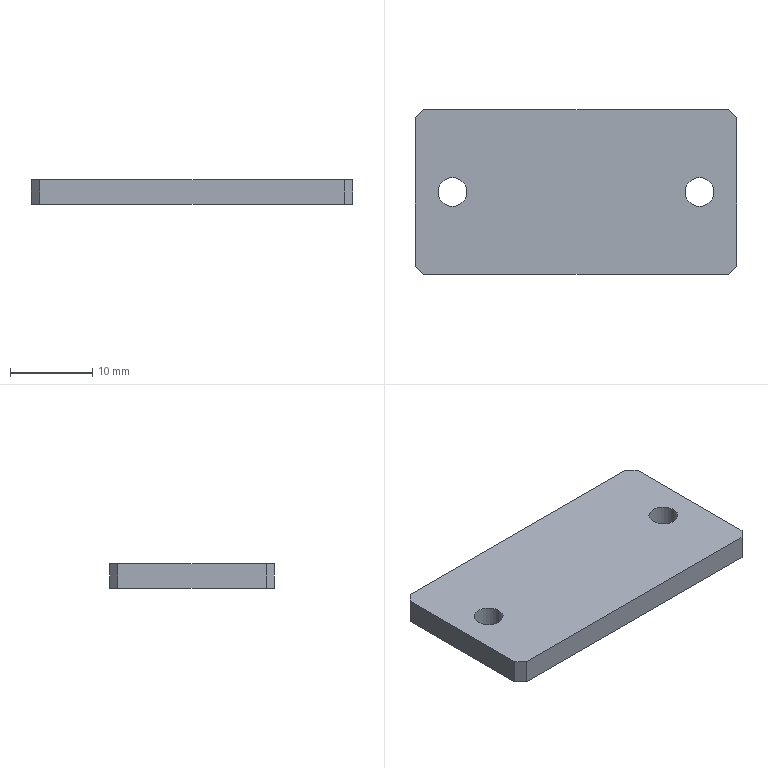Part | SolidWorks | features Chamfer 1, Extrusion 1 | 1 solid | 14 faces | box 39 x 20 x 3 mm | volume 2276 mm3 | plane 10 | cylinder 4 | commonest cylinder face diameters 3.5 x4
STEP:
#1=CARTESIAN_POINT('',(13.25,0.,3.));
#2=VERTEX_POINT('',#1);
#3=CARTESIAN_POINT('',(16.75,0.,3.));
#4=VERTEX_POINT('',#3);
#5=CARTESIAN_POINT('',(15.,0.,3.));
#6=DIRECTION('',(0.,0.,1.));
#7=DIRECTION('',(1.,0.,0.));
#8=AXIS2_PLACEMENT_3D('',#5,#6,#7);
#9=CIRCLE('',#8,1.75);
#10=EDGE_CURVE('',#2,#4,#9,.T.);
#11=ORIENTED_EDGE('',*,*,#10,.T.);
#12=CARTESIAN_POINT('',(16.75,0.,0.));
#13=VERTEX_POINT('',#12);
#14=CARTESIAN_POINT('',(16.75,0.,3.));
#15=DIRECTION('',(0.,0.,-1.));
#16=VECTOR('',#15,1000.);
#17=LINE('',#14,#16);
#18=EDGE_CURVE('',#4,#13,#17,.T.);
#19=ORIENTED_EDGE('',*,*,#18,.T.);
#20=CARTESIAN_POINT('',(13.25,0.,0.));
#21=VERTEX_POINT('',#20);
#22=CARTESIAN_POINT('',(15.,0.,0.));
#23=DIRECTION('',(0.,0.,1.));
#24=DIRECTION('',(1.,0.,0.));
#25=AXIS2_PLACEMENT_3D('',#22,#23,#24);
#26=CIRCLE('',#25,1.75);
#27=EDGE_CURVE('',#21,#13,#26,.T.);
#28=ORIENTED_EDGE('',*,*,#27,.F.);
#29=CARTESIAN_POINT('',(13.25,0.,3.));
#30=DIRECTION('',(0.,0.,-1.));
#31=VECTOR('',#30,1000.);
#32=LINE('',#29,#31);
#33=EDGE_CURVE('',#2,#21,#32,.T.);
#34=ORIENTED_EDGE('',*,*,#33,.F.);
#35=EDGE_LOOP('',(#11,#19,#28,#34));
#36=FACE_OUTER_BOUND('',#35,.T.);
#37=CARTESIAN_POINT('',(15.,0.,3.));
#38=DIRECTION('',(0.,0.,-1.));
#39=DIRECTION('',(-1.,0.,0.));
#40=AXIS2_PLACEMENT_3D('',#37,#38,#39);
#41=CYLINDRICAL_SURFACE('',#40,1.75);
#42=ADVANCED_FACE('',(#36),#41,.F.);
#43=CARTESIAN_POINT('',(-16.75,0.,3.));
#44=VERTEX_POINT('',#43);
#45=CARTESIAN_POINT('',(-13.25,0.,3.));
#46=VERTEX_POINT('',#45);
#47=CARTESIAN_POINT('',(-15.,0.,3.));
#48=DIRECTION('',(0.,0.,1.));
#49=DIRECTION('',(1.,0.,0.));
#50=AXIS2_PLACEMENT_3D('',#47,#48,#49);
#51=CIRCLE('',#50,1.75);
#52=EDGE_CURVE('',#44,#46,#51,.T.);
#53=ORIENTED_EDGE('',*,*,#52,.T.);
#54=CARTESIAN_POINT('',(-13.25,0.,0.));
#55=VERTEX_POINT('',#54);
#56=CARTESIAN_POINT('',(-13.25,0.,3.));
#57=DIRECTION('',(0.,0.,-1.));
#58=VECTOR('',#57,1000.);
#59=LINE('',#56,#58);
#60=EDGE_CURVE('',#46,#55,#59,.T.);
#61=ORIENTED_EDGE('',*,*,#60,.T.);
#62=CARTESIAN_POINT('',(-16.75,0.,0.));
#63=VERTEX_POINT('',#62);
#64=CARTESIAN_POINT('',(-15.,0.,0.));
#65=DIRECTION('',(0.,0.,1.));
#66=DIRECTION('',(1.,0.,0.));
#67=AXIS2_PLACEMENT_3D('',#64,#65,#66);
#68=CIRCLE('',#67,1.75);
#69=EDGE_CURVE('',#63,#55,#68,.T.);
#70=ORIENTED_EDGE('',*,*,#69,.F.);
#71=CARTESIAN_POINT('',(-16.75,0.,3.));
#72=DIRECTION('',(0.,0.,-1.));
#73=VECTOR('',#72,1000.);
#74=LINE('',#71,#73);
#75=EDGE_CURVE('',#44,#63,#74,.T.);
#76=ORIENTED_EDGE('',*,*,#75,.F.);
#77=EDGE_LOOP('',(#53,#61,#70,#76));
#78=FACE_OUTER_BOUND('',#77,.T.);
#79=CARTESIAN_POINT('',(-15.,0.,3.));
#80=DIRECTION('',(0.,0.,-1.));
#81=DIRECTION('',(-1.,0.,0.));
#82=AXIS2_PLACEMENT_3D('',#79,#80,#81);
#83=CYLINDRICAL_SURFACE('',#82,1.75);
#84=ADVANCED_FACE('',(#78),#83,.F.);
#85=CARTESIAN_POINT('',(-18.5,-10.,3.));
#86=VERTEX_POINT('',#85);
#87=CARTESIAN_POINT('',(18.5,-10.,3.));
#88=VERTEX_POINT('',#87);
#89=CARTESIAN_POINT('',(-19.5,-10.,3.));
#90=DIRECTION('',(1.,0.,0.));
#91=VECTOR('',#90,1000.);
#92=LINE('',#89,#91);
#93=EDGE_CURVE('',#86,#88,#92,.T.);
#94=ORIENTED_EDGE('',*,*,#93,.T.);
#95=CARTESIAN_POINT('',(19.5,-9.,3.));
#96=VERTEX_POINT('',#95);
#97=CARTESIAN_POINT('',(19.5,-9.,3.));
#98=DIRECTION('',(0.7071,0.7071,0.));
#99=VECTOR('',#98,1000.);
#100=LINE('',#97,#99);
#101=EDGE_CURVE('',#88,#96,#100,.T.);
#102=ORIENTED_EDGE('',*,*,#101,.T.);
#103=CARTESIAN_POINT('',(19.5,9.,3.));
#104=VERTEX_POINT('',#103);
#105=CARTESIAN_POINT('',(19.5,-10.,3.));
#106=DIRECTION('',(0.,1.,0.));
#107=VECTOR('',#106,1000.);
#108=LINE('',#105,#107);
#109=EDGE_CURVE('',#96,#104,#108,.T.);
#110=ORIENTED_EDGE('',*,*,#109,.T.);
#111=CARTESIAN_POINT('',(18.5,10.,3.));
#112=VERTEX_POINT('',#111);
#113=CARTESIAN_POINT('',(18.5,10.,3.));
#114=DIRECTION('',(-0.7071,0.7071,0.));
#115=VECTOR('',#114,1000.);
#116=LINE('',#113,#115);
#117=EDGE_CURVE('',#104,#112,#116,.T.);
#118=ORIENTED_EDGE('',*,*,#117,.T.);
#119=CARTESIAN_POINT('',(-18.5,10.,3.));
#120=VERTEX_POINT('',#119);
#121=CARTESIAN_POINT('',(-19.5,10.,3.));
#122=DIRECTION('',(-1.,0.,0.));
#123=VECTOR('',#122,1000.);
#124=LINE('',#121,#123);
#125=EDGE_CURVE('',#112,#120,#124,.T.);
#126=ORIENTED_EDGE('',*,*,#125,.T.);
#127=CARTESIAN_POINT('',(-19.5,9.,3.));
#128=VERTEX_POINT('',#127);
#129=CARTESIAN_POINT('',(-19.5,9.,3.));
#130=DIRECTION('',(-0.7071,-0.7071,0.));
#131=VECTOR('',#130,1000.);
#132=LINE('',#129,#131);
#133=EDGE_CURVE('',#120,#128,#132,.T.);
#134=ORIENTED_EDGE('',*,*,#133,.T.);
#135=CARTESIAN_POINT('',(-19.5,-9.,3.));
#136=VERTEX_POINT('',#135);
#137=CARTESIAN_POINT('',(-19.5,-10.,3.));
#138=DIRECTION('',(0.,-1.,0.));
#139=VECTOR('',#138,1000.);
#140=LINE('',#137,#139);
#141=EDGE_CURVE('',#128,#136,#140,.T.);
#142=ORIENTED_EDGE('',*,*,#141,.T.);
#143=CARTESIAN_POINT('',(-18.5,-10.,3.));
#144=DIRECTION('',(0.7071,-0.7071,0.));
#145=VECTOR('',#144,1000.);
#146=LINE('',#143,#145);
#147=EDGE_CURVE('',#136,#86,#146,.T.);
#148=ORIENTED_EDGE('',*,*,#147,.T.);
#149=EDGE_LOOP('',(#94,#102,#110,#118,#126,#134,#142,#148));
#150=FACE_OUTER_BOUND('',#149,.T.);
#151=ORIENTED_EDGE('',*,*,#52,.F.);
#152=CARTESIAN_POINT('',(-15.,0.,3.));
#153=DIRECTION('',(0.,0.,1.));
#154=DIRECTION('',(1.,0.,0.));
#155=AXIS2_PLACEMENT_3D('',#152,#153,#154);
#156=CIRCLE('',#155,1.75);
#157=EDGE_CURVE('',#46,#44,#156,.T.);
#158=ORIENTED_EDGE('',*,*,#157,.F.);
#159=EDGE_LOOP('',(#151,#158));
#160=FACE_BOUND('',#159,.T.);
#161=ORIENTED_EDGE('',*,*,#10,.F.);
#162=CARTESIAN_POINT('',(15.,0.,3.));
#163=DIRECTION('',(0.,0.,1.));
#164=DIRECTION('',(1.,0.,0.));
#165=AXIS2_PLACEMENT_3D('',#162,#163,#164);
#166=CIRCLE('',#165,1.75);
#167=EDGE_CURVE('',#4,#2,#166,.T.);
#168=ORIENTED_EDGE('',*,*,#167,.F.);
#169=EDGE_LOOP('',(#161,#168));
#170=FACE_BOUND('',#169,.T.);
#171=CARTESIAN_POINT('',(0.,0.,3.));
#172=DIRECTION('',(0.,0.,-1.));
#173=DIRECTION('',(-1.,0.,0.));
#174=AXIS2_PLACEMENT_3D('',#171,#172,#173);
#175=PLANE('',#174);
#176=ADVANCED_FACE('',(#150,#160,#170),#175,.F.);
#177=ORIENTED_EDGE('',*,*,#69,.T.);
#178=CARTESIAN_POINT('',(-15.,0.,0.));
#179=DIRECTION('',(0.,0.,1.));
#180=DIRECTION('',(1.,0.,0.));
#181=AXIS2_PLACEMENT_3D('',#178,#179,#180);
#182=CIRCLE('',#181,1.75);
#183=EDGE_CURVE('',#55,#63,#182,.T.);
#184=ORIENTED_EDGE('',*,*,#183,.T.);
#185=EDGE_LOOP('',(#177,#184));
#186=FACE_BOUND('',#185,.T.);
#187=CARTESIAN_POINT('',(19.5,-9.,0.));
#188=VERTEX_POINT('',#187);
#189=CARTESIAN_POINT('',(19.5,9.,0.));
#190=VERTEX_POINT('',#189);
#191=CARTESIAN_POINT('',(19.5,-10.,0.));
#192=DIRECTION('',(0.,1.,0.));
#193=VECTOR('',#192,1000.);
#194=LINE('',#191,#193);
#195=EDGE_CURVE('',#188,#190,#194,.T.);
#196=ORIENTED_EDGE('',*,*,#195,.F.);
#197=CARTESIAN_POINT('',(18.5,-10.,0.));
#198=VERTEX_POINT('',#197);
#199=CARTESIAN_POINT('',(14.25,-14.25,0.));
#200=DIRECTION('',(-0.7071,-0.7071,0.));
#201=VECTOR('',#200,1000.);
#202=LINE('',#199,#201);
#203=EDGE_CURVE('',#188,#198,#202,.T.);
#204=ORIENTED_EDGE('',*,*,#203,.T.);
#205=CARTESIAN_POINT('',(-18.5,-10.,0.));
#206=VERTEX_POINT('',#205);
#207=CARTESIAN_POINT('',(-19.5,-10.,0.));
#208=DIRECTION('',(1.,0.,0.));
#209=VECTOR('',#208,1000.);
#210=LINE('',#207,#209);
#211=EDGE_CURVE('',#206,#198,#210,.T.);
#212=ORIENTED_EDGE('',*,*,#211,.F.);
#213=CARTESIAN_POINT('',(-19.5,-9.,0.));
#214=VERTEX_POINT('',#213);
#215=CARTESIAN_POINT('',(-14.25,-14.25,0.));
#216=DIRECTION('',(-0.7071,0.7071,0.));
#217=VECTOR('',#216,1000.);
#218=LINE('',#215,#217);
#219=EDGE_CURVE('',#206,#214,#218,.T.);
#220=ORIENTED_EDGE('',*,*,#219,.T.);
#221=CARTESIAN_POINT('',(-19.5,9.,0.));
#222=VERTEX_POINT('',#221);
#223=CARTESIAN_POINT('',(-19.5,-10.,0.));
#224=DIRECTION('',(0.,-1.,0.));
#225=VECTOR('',#224,1000.);
#226=LINE('',#223,#225);
#227=EDGE_CURVE('',#222,#214,#226,.T.);
#228=ORIENTED_EDGE('',*,*,#227,.F.);
#229=CARTESIAN_POINT('',(-18.5,10.,0.));
#230=VERTEX_POINT('',#229);
#231=CARTESIAN_POINT('',(-14.25,14.25,0.));
#232=DIRECTION('',(0.7071,0.7071,0.));
#233=VECTOR('',#232,1000.);
#234=LINE('',#231,#233);
#235=EDGE_CURVE('',#222,#230,#234,.T.);
#236=ORIENTED_EDGE('',*,*,#235,.T.);
#237=CARTESIAN_POINT('',(18.5,10.,0.));
#238=VERTEX_POINT('',#237);
#239=CARTESIAN_POINT('',(-19.5,10.,0.));
#240=DIRECTION('',(-1.,0.,0.));
#241=VECTOR('',#240,1000.);
#242=LINE('',#239,#241);
#243=EDGE_CURVE('',#238,#230,#242,.T.);
#244=ORIENTED_EDGE('',*,*,#243,.F.);
#245=CARTESIAN_POINT('',(14.25,14.25,0.));
#246=DIRECTION('',(0.7071,-0.7071,0.));
#247=VECTOR('',#246,1000.);
#248=LINE('',#245,#247);
#249=EDGE_CURVE('',#238,#190,#248,.T.);
#250=ORIENTED_EDGE('',*,*,#249,.T.);
#251=EDGE_LOOP('',(#196,#204,#212,#220,#228,#236,#244,#250));
#252=FACE_OUTER_BOUND('',#251,.T.);
#253=ORIENTED_EDGE('',*,*,#27,.T.);
#254=CARTESIAN_POINT('',(15.,0.,0.));
#255=DIRECTION('',(0.,0.,1.));
#256=DIRECTION('',(1.,0.,0.));
#257=AXIS2_PLACEMENT_3D('',#254,#255,#256);
#258=CIRCLE('',#257,1.75);
#259=EDGE_CURVE('',#13,#21,#258,.T.);
#260=ORIENTED_EDGE('',*,*,#259,.T.);
#261=EDGE_LOOP('',(#253,#260));
#262=FACE_BOUND('',#261,.T.);
#263=CARTESIAN_POINT('',(0.,0.,0.));
#264=DIRECTION('',(0.,0.,-1.));
#265=DIRECTION('',(-1.,0.,0.));
#266=AXIS2_PLACEMENT_3D('',#263,#264,#265);
#267=PLANE('',#266);
#268=ADVANCED_FACE('',(#186,#252,#262),#267,.T.);
#269=ORIENTED_EDGE('',*,*,#109,.F.);
#270=CARTESIAN_POINT('',(19.5,-9.,3.));
#271=DIRECTION('',(0.,0.,-1.));
#272=VECTOR('',#271,1000.);
#273=LINE('',#270,#272);
#274=EDGE_CURVE('',#96,#188,#273,.T.);
#275=ORIENTED_EDGE('',*,*,#274,.T.);
#276=ORIENTED_EDGE('',*,*,#195,.T.);
#277=CARTESIAN_POINT('',(19.5,9.,3.));
#278=DIRECTION('',(0.,0.,1.));
#279=VECTOR('',#278,1000.);
#280=LINE('',#277,#279);
#281=EDGE_CURVE('',#190,#104,#280,.T.);
#282=ORIENTED_EDGE('',*,*,#281,.T.);
#283=EDGE_LOOP('',(#269,#275,#276,#282));
#284=FACE_OUTER_BOUND('',#283,.T.);
#285=CARTESIAN_POINT('',(19.5,-10.,3.));
#286=DIRECTION('',(-1.,0.,0.));
#287=DIRECTION('',(0.,-1.,0.));
#288=AXIS2_PLACEMENT_3D('',#285,#286,#287);
#289=PLANE('',#288);
#290=ADVANCED_FACE('',(#284),#289,.F.);
#291=ORIENTED_EDGE('',*,*,#125,.F.);
#292=CARTESIAN_POINT('',(18.5,10.,3.));
#293=DIRECTION('',(0.,0.,-1.));
#294=VECTOR('',#293,1000.);
#295=LINE('',#292,#294);
#296=EDGE_CURVE('',#112,#238,#295,.T.);
#297=ORIENTED_EDGE('',*,*,#296,.T.);
#298=ORIENTED_EDGE('',*,*,#243,.T.);
#299=CARTESIAN_POINT('',(-18.5,10.,3.));
#300=DIRECTION('',(0.,0.,1.));
#301=VECTOR('',#300,1000.);
#302=LINE('',#299,#301);
#303=EDGE_CURVE('',#230,#120,#302,.T.);
#304=ORIENTED_EDGE('',*,*,#303,.T.);
#305=EDGE_LOOP('',(#291,#297,#298,#304));
#306=FACE_OUTER_BOUND('',#305,.T.);
#307=CARTESIAN_POINT('',(-19.5,10.,3.));
#308=DIRECTION('',(0.,-1.,0.));
#309=DIRECTION('',(1.,0.,0.));
#310=AXIS2_PLACEMENT_3D('',#307,#308,#309);
#311=PLANE('',#310);
#312=ADVANCED_FACE('',(#306),#311,.F.);
#313=ORIENTED_EDGE('',*,*,#227,.T.);
#314=CARTESIAN_POINT('',(-19.5,-9.,3.));
#315=DIRECTION('',(0.,0.,1.));
#316=VECTOR('',#315,1000.);
#317=LINE('',#314,#316);
#318=EDGE_CURVE('',#214,#136,#317,.T.);
#319=ORIENTED_EDGE('',*,*,#318,.T.);
#320=ORIENTED_EDGE('',*,*,#141,.F.);
#321=CARTESIAN_POINT('',(-19.5,9.,3.));
#322=DIRECTION('',(0.,0.,-1.));
#323=VECTOR('',#322,1000.);
#324=LINE('',#321,#323);
#325=EDGE_CURVE('',#128,#222,#324,.T.);
#326=ORIENTED_EDGE('',*,*,#325,.T.);
#327=EDGE_LOOP('',(#313,#319,#320,#326));
#328=FACE_OUTER_BOUND('',#327,.T.);
#329=CARTESIAN_POINT('',(-19.5,-10.,3.));
#330=DIRECTION('',(1.,0.,0.));
#331=DIRECTION('',(0.,0.,-1.));
#332=AXIS2_PLACEMENT_3D('',#329,#330,#331);
#333=PLANE('',#332);
#334=ADVANCED_FACE('',(#328),#333,.F.);
#335=ORIENTED_EDGE('',*,*,#211,.T.);
#336=CARTESIAN_POINT('',(18.5,-10.,3.));
#337=DIRECTION('',(0.,0.,1.));
#338=VECTOR('',#337,1000.);
#339=LINE('',#336,#338);
#340=EDGE_CURVE('',#198,#88,#339,.T.);
#341=ORIENTED_EDGE('',*,*,#340,.T.);
#342=ORIENTED_EDGE('',*,*,#93,.F.);
#343=CARTESIAN_POINT('',(-18.5,-10.,3.));
#344=DIRECTION('',(0.,0.,-1.));
#345=VECTOR('',#344,1000.);
#346=LINE('',#343,#345);
#347=EDGE_CURVE('',#86,#206,#346,.T.);
#348=ORIENTED_EDGE('',*,*,#347,.T.);
#349=EDGE_LOOP('',(#335,#341,#342,#348));
#350=FACE_OUTER_BOUND('',#349,.T.);
#351=CARTESIAN_POINT('',(-19.5,-10.,3.));
#352=DIRECTION('',(0.,1.,0.));
#353=DIRECTION('',(0.,0.,1.));
#354=AXIS2_PLACEMENT_3D('',#351,#352,#353);
#355=PLANE('',#354);
#356=ADVANCED_FACE('',(#350),#355,.F.);
#357=ORIENTED_EDGE('',*,*,#60,.F.);
#358=ORIENTED_EDGE('',*,*,#157,.T.);
#359=ORIENTED_EDGE('',*,*,#75,.T.);
#360=ORIENTED_EDGE('',*,*,#183,.F.);
#361=EDGE_LOOP('',(#357,#358,#359,#360));
#362=FACE_OUTER_BOUND('',#361,.T.);
#363=CARTESIAN_POINT('',(-15.,0.,3.));
#364=DIRECTION('',(0.,0.,-1.));
#365=DIRECTION('',(-1.,0.,0.));
#366=AXIS2_PLACEMENT_3D('',#363,#364,#365);
#367=CYLINDRICAL_SURFACE('',#366,1.75);
#368=ADVANCED_FACE('',(#362),#367,.F.);
#369=ORIENTED_EDGE('',*,*,#18,.F.);
#370=ORIENTED_EDGE('',*,*,#167,.T.);
#371=ORIENTED_EDGE('',*,*,#33,.T.);
#372=ORIENTED_EDGE('',*,*,#259,.F.);
#373=EDGE_LOOP('',(#369,#370,#371,#372));
#374=FACE_OUTER_BOUND('',#373,.T.);
#375=CARTESIAN_POINT('',(15.,0.,3.));
#376=DIRECTION('',(0.,0.,-1.));
#377=DIRECTION('',(-1.,0.,0.));
#378=AXIS2_PLACEMENT_3D('',#375,#376,#377);
#379=CYLINDRICAL_SURFACE('',#378,1.75);
#380=ADVANCED_FACE('',(#374),#379,.F.);
#381=ORIENTED_EDGE('',*,*,#101,.F.);
#382=ORIENTED_EDGE('',*,*,#340,.F.);
#383=ORIENTED_EDGE('',*,*,#203,.F.);
#384=ORIENTED_EDGE('',*,*,#274,.F.);
#385=EDGE_LOOP('',(#381,#382,#383,#384));
#386=FACE_OUTER_BOUND('',#385,.T.);
#387=CARTESIAN_POINT('',(19.5,-9.,3.));
#388=DIRECTION('',(-0.7071,0.7071,0.));
#389=DIRECTION('',(0.,0.,-1.));
#390=AXIS2_PLACEMENT_3D('',#387,#388,#389);
#391=PLANE('',#390);
#392=ADVANCED_FACE('',(#386),#391,.F.);
#393=ORIENTED_EDGE('',*,*,#117,.F.);
#394=ORIENTED_EDGE('',*,*,#281,.F.);
#395=ORIENTED_EDGE('',*,*,#249,.F.);
#396=ORIENTED_EDGE('',*,*,#296,.F.);
#397=EDGE_LOOP('',(#393,#394,#395,#396));
#398=FACE_OUTER_BOUND('',#397,.T.);
#399=CARTESIAN_POINT('',(18.5,10.,3.));
#400=DIRECTION('',(-0.7071,-0.7071,0.));
#401=DIRECTION('',(0.,0.,-1.));
#402=AXIS2_PLACEMENT_3D('',#399,#400,#401);
#403=PLANE('',#402);
#404=ADVANCED_FACE('',(#398),#403,.F.);
#405=ORIENTED_EDGE('',*,*,#147,.F.);
#406=ORIENTED_EDGE('',*,*,#318,.F.);
#407=ORIENTED_EDGE('',*,*,#219,.F.);
#408=ORIENTED_EDGE('',*,*,#347,.F.);
#409=EDGE_LOOP('',(#405,#406,#407,#408));
#410=FACE_OUTER_BOUND('',#409,.T.);
#411=CARTESIAN_POINT('',(-18.5,-10.,3.));
#412=DIRECTION('',(0.7071,0.7071,0.));
#413=DIRECTION('',(0.,0.,-1.));
#414=AXIS2_PLACEMENT_3D('',#411,#412,#413);
#415=PLANE('',#414);
#416=ADVANCED_FACE('',(#410),#415,.F.);
#417=ORIENTED_EDGE('',*,*,#133,.F.);
#418=ORIENTED_EDGE('',*,*,#303,.F.);
#419=ORIENTED_EDGE('',*,*,#235,.F.);
#420=ORIENTED_EDGE('',*,*,#325,.F.);
#421=EDGE_LOOP('',(#417,#418,#419,#420));
#422=FACE_OUTER_BOUND('',#421,.T.);
#423=CARTESIAN_POINT('',(-19.5,9.,3.));
#424=DIRECTION('',(0.7071,-0.7071,0.));
#425=DIRECTION('',(0.,0.,-1.));
#426=AXIS2_PLACEMENT_3D('',#423,#424,#425);
#427=PLANE('',#426);
#428=ADVANCED_FACE('',(#422),#427,.F.);
#429=CLOSED_SHELL('',(#42,#84,#176,#268,#290,#312,#334,#356,#368,#380,#392,#404,#416,#428));
#430=MANIFOLD_SOLID_BREP('',#429);
#431=CARTESIAN_POINT('',(0.,0.,0.));
#432=DIRECTION('',(0.,0.,1.));
#433=DIRECTION('',(1.,0.,0.));
#434=AXIS2_PLACEMENT_3D('',#431,#432,#433);
#435=(LENGTH_UNIT()NAMED_UNIT(*)SI_UNIT(.MILLI.,.METRE.));
#436=UNCERTAINTY_MEASURE_WITH_UNIT(LENGTH_MEASURE(0.00001),#435,'','');
#437=(NAMED_UNIT(*)PLANE_ANGLE_UNIT()SI_UNIT($,.RADIAN.));
#438=(NAMED_UNIT(*)SI_UNIT($,.STERADIAN.)SOLID_ANGLE_UNIT());
#439=(GEOMETRIC_REPRESENTATION_CONTEXT(3)GLOBAL_UNCERTAINTY_ASSIGNED_CONTEXT((#436))GLOBAL_UNIT_ASSIGNED_CONTEXT((#435,#437,#438))REPRESENTATION_CONTEXT('',''));
#440=ADVANCED_BREP_SHAPE_REPRESENTATION('',(#430,#434),#439);